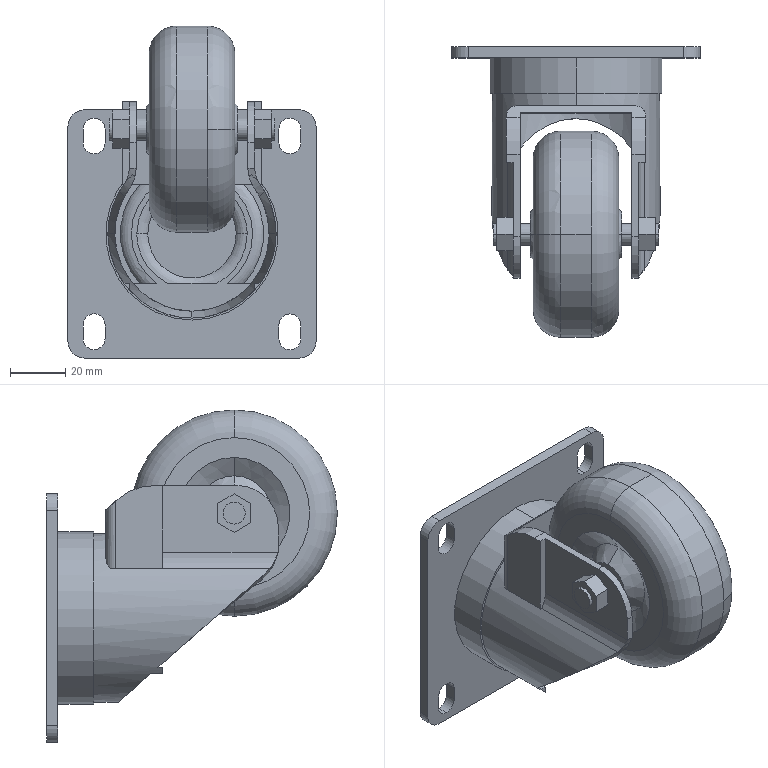Part | NX | features BREP 1 | 1 solid | 140 faces | box 90 x 105.39 x 120.39 mm | volume 234648 mm3 | plane 69 | cylinder 47 | cone 8 | torus 8 | spline 8 | commonest cylinder face diameters 8 x20 9 x4 12 x4 61 x4 7 x2 20 x2